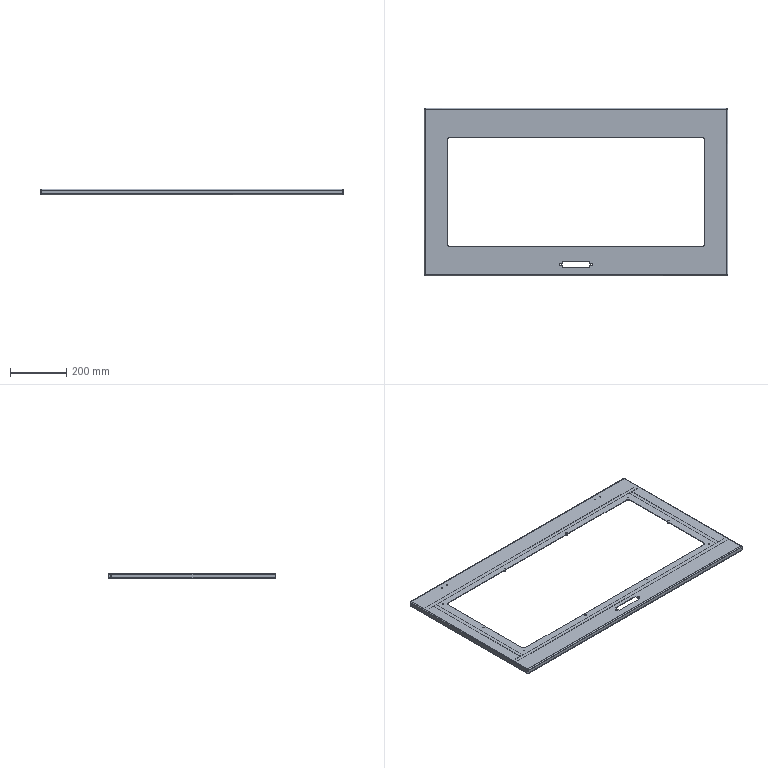Part | NX | features BREP 5 | 5 solids | 264 faces | box 1078 x 595 x 20 mm | volume 937923 mm3 | plane 144 | cylinder 76 | cone 28 | spline 16 | commonest cylinder face diameters 5 x20 4 x18 8 x14 6 x8 7 x8 6.5 x4